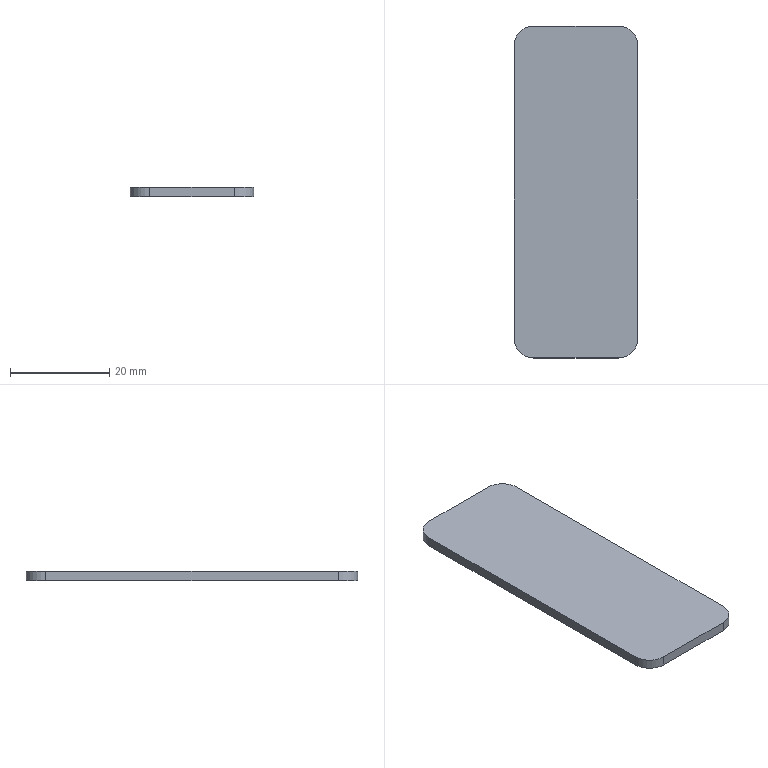Part | STEP file | X77-08306 | 1 solid | 10 faces | box 25 x 67 x 2 mm | volume 3323 mm3 | plane 6 | cylinder 4 | commonest cylinder face diameters 8 x4
STEP:
#1=CARTESIAN_POINT('',(-8.5,622.876,0.));
#2=VERTEX_POINT('',#1);
#3=CARTESIAN_POINT('',(-12.5,618.876,0.));
#4=VERTEX_POINT('',#3);
#5=CARTESIAN_POINT('',(-8.5,618.876,0.));
#6=DIRECTION('',(0.,0.,1.));
#7=DIRECTION('',(1.,0.,0.));
#8=AXIS2_PLACEMENT_3D('',#5,#6,#7);
#9=CIRCLE('',#8,4.);
#10=EDGE_CURVE('',#2,#4,#9,.T.);
#11=ORIENTED_EDGE('',*,*,#10,.T.);
#12=CARTESIAN_POINT('',(-12.5,618.876,2.));
#13=VERTEX_POINT('',#12);
#14=CARTESIAN_POINT('',(-12.5,618.876,2.));
#15=DIRECTION('',(0.,0.,-1.));
#16=VECTOR('',#15,1000.);
#17=LINE('',#14,#16);
#18=EDGE_CURVE('',#13,#4,#17,.T.);
#19=ORIENTED_EDGE('',*,*,#18,.F.);
#20=CARTESIAN_POINT('',(-8.5,622.876,2.));
#21=VERTEX_POINT('',#20);
#22=CARTESIAN_POINT('',(-8.5,618.876,2.));
#23=DIRECTION('',(0.,0.,1.));
#24=DIRECTION('',(1.,0.,0.));
#25=AXIS2_PLACEMENT_3D('',#22,#23,#24);
#26=CIRCLE('',#25,4.);
#27=EDGE_CURVE('',#21,#13,#26,.T.);
#28=ORIENTED_EDGE('',*,*,#27,.F.);
#29=CARTESIAN_POINT('',(-8.5,622.876,2.));
#30=DIRECTION('',(0.,0.,-1.));
#31=VECTOR('',#30,1000.);
#32=LINE('',#29,#31);
#33=EDGE_CURVE('',#21,#2,#32,.T.);
#34=ORIENTED_EDGE('',*,*,#33,.T.);
#35=EDGE_LOOP('',(#11,#19,#28,#34));
#36=FACE_OUTER_BOUND('',#35,.T.);
#37=CARTESIAN_POINT('',(-8.5,618.876,2.));
#38=DIRECTION('',(0.,0.,-1.));
#39=DIRECTION('',(-1.,0.,0.));
#40=AXIS2_PLACEMENT_3D('',#37,#38,#39);
#41=CYLINDRICAL_SURFACE('',#40,4.);
#42=ADVANCED_FACE('',(#36),#41,.T.);
#43=CARTESIAN_POINT('',(-12.5,559.876,0.));
#44=VERTEX_POINT('',#43);
#45=CARTESIAN_POINT('',(-12.5,618.876,0.));
#46=DIRECTION('',(0.,-1.,0.));
#47=VECTOR('',#46,1000.);
#48=LINE('',#45,#47);
#49=EDGE_CURVE('',#4,#44,#48,.T.);
#50=ORIENTED_EDGE('',*,*,#49,.T.);
#51=CARTESIAN_POINT('',(-12.5,559.876,2.));
#52=VERTEX_POINT('',#51);
#53=CARTESIAN_POINT('',(-12.5,559.876,2.));
#54=DIRECTION('',(0.,0.,-1.));
#55=VECTOR('',#54,1000.);
#56=LINE('',#53,#55);
#57=EDGE_CURVE('',#52,#44,#56,.T.);
#58=ORIENTED_EDGE('',*,*,#57,.F.);
#59=CARTESIAN_POINT('',(-12.5,618.876,2.));
#60=DIRECTION('',(0.,-1.,0.));
#61=VECTOR('',#60,1000.);
#62=LINE('',#59,#61);
#63=EDGE_CURVE('',#13,#52,#62,.T.);
#64=ORIENTED_EDGE('',*,*,#63,.F.);
#65=ORIENTED_EDGE('',*,*,#18,.T.);
#66=EDGE_LOOP('',(#50,#58,#64,#65));
#67=FACE_OUTER_BOUND('',#66,.T.);
#68=CARTESIAN_POINT('',(-12.5,618.876,2.));
#69=DIRECTION('',(1.,0.,0.));
#70=DIRECTION('',(0.,0.,-1.));
#71=AXIS2_PLACEMENT_3D('',#68,#69,#70);
#72=PLANE('',#71);
#73=ADVANCED_FACE('',(#67),#72,.F.);
#74=CARTESIAN_POINT('',(-8.5,555.876,0.));
#75=VERTEX_POINT('',#74);
#76=CARTESIAN_POINT('',(-8.5,559.876,0.));
#77=DIRECTION('',(0.,0.,1.));
#78=DIRECTION('',(1.,0.,0.));
#79=AXIS2_PLACEMENT_3D('',#76,#77,#78);
#80=CIRCLE('',#79,4.);
#81=EDGE_CURVE('',#44,#75,#80,.T.);
#82=ORIENTED_EDGE('',*,*,#81,.T.);
#83=CARTESIAN_POINT('',(-8.5,555.876,2.));
#84=VERTEX_POINT('',#83);
#85=CARTESIAN_POINT('',(-8.5,555.876,2.));
#86=DIRECTION('',(0.,0.,-1.));
#87=VECTOR('',#86,1000.);
#88=LINE('',#85,#87);
#89=EDGE_CURVE('',#84,#75,#88,.T.);
#90=ORIENTED_EDGE('',*,*,#89,.F.);
#91=CARTESIAN_POINT('',(-8.5,559.876,2.));
#92=DIRECTION('',(0.,0.,1.));
#93=DIRECTION('',(1.,0.,0.));
#94=AXIS2_PLACEMENT_3D('',#91,#92,#93);
#95=CIRCLE('',#94,4.);
#96=EDGE_CURVE('',#52,#84,#95,.T.);
#97=ORIENTED_EDGE('',*,*,#96,.F.);
#98=ORIENTED_EDGE('',*,*,#57,.T.);
#99=EDGE_LOOP('',(#82,#90,#97,#98));
#100=FACE_OUTER_BOUND('',#99,.T.);
#101=CARTESIAN_POINT('',(-8.5,559.876,2.));
#102=DIRECTION('',(0.,0.,-1.));
#103=DIRECTION('',(-1.,0.,0.));
#104=AXIS2_PLACEMENT_3D('',#101,#102,#103);
#105=CYLINDRICAL_SURFACE('',#104,4.);
#106=ADVANCED_FACE('',(#100),#105,.T.);
#107=CARTESIAN_POINT('',(8.5,555.876,0.));
#108=VERTEX_POINT('',#107);
#109=CARTESIAN_POINT('',(-8.5,555.876,0.));
#110=DIRECTION('',(1.,0.,0.));
#111=VECTOR('',#110,1000.);
#112=LINE('',#109,#111);
#113=EDGE_CURVE('',#75,#108,#112,.T.);
#114=ORIENTED_EDGE('',*,*,#113,.T.);
#115=CARTESIAN_POINT('',(8.5,555.876,2.));
#116=VERTEX_POINT('',#115);
#117=CARTESIAN_POINT('',(8.5,555.876,2.));
#118=DIRECTION('',(0.,0.,-1.));
#119=VECTOR('',#118,1000.);
#120=LINE('',#117,#119);
#121=EDGE_CURVE('',#116,#108,#120,.T.);
#122=ORIENTED_EDGE('',*,*,#121,.F.);
#123=CARTESIAN_POINT('',(-8.5,555.876,2.));
#124=DIRECTION('',(1.,0.,0.));
#125=VECTOR('',#124,1000.);
#126=LINE('',#123,#125);
#127=EDGE_CURVE('',#84,#116,#126,.T.);
#128=ORIENTED_EDGE('',*,*,#127,.F.);
#129=ORIENTED_EDGE('',*,*,#89,.T.);
#130=EDGE_LOOP('',(#114,#122,#128,#129));
#131=FACE_OUTER_BOUND('',#130,.T.);
#132=CARTESIAN_POINT('',(-8.5,555.876,2.));
#133=DIRECTION('',(0.,1.,0.));
#134=DIRECTION('',(0.,0.,1.));
#135=AXIS2_PLACEMENT_3D('',#132,#133,#134);
#136=PLANE('',#135);
#137=ADVANCED_FACE('',(#131),#136,.F.);
#138=CARTESIAN_POINT('',(12.5,559.876,0.));
#139=VERTEX_POINT('',#138);
#140=CARTESIAN_POINT('',(8.5,559.876,0.));
#141=DIRECTION('',(0.,0.,1.));
#142=DIRECTION('',(1.,0.,0.));
#143=AXIS2_PLACEMENT_3D('',#140,#141,#142);
#144=CIRCLE('',#143,4.);
#145=EDGE_CURVE('',#108,#139,#144,.T.);
#146=ORIENTED_EDGE('',*,*,#145,.T.);
#147=CARTESIAN_POINT('',(12.5,559.876,2.));
#148=VERTEX_POINT('',#147);
#149=CARTESIAN_POINT('',(12.5,559.876,2.));
#150=DIRECTION('',(0.,0.,-1.));
#151=VECTOR('',#150,1000.);
#152=LINE('',#149,#151);
#153=EDGE_CURVE('',#148,#139,#152,.T.);
#154=ORIENTED_EDGE('',*,*,#153,.F.);
#155=CARTESIAN_POINT('',(8.5,559.876,2.));
#156=DIRECTION('',(0.,0.,1.));
#157=DIRECTION('',(1.,0.,0.));
#158=AXIS2_PLACEMENT_3D('',#155,#156,#157);
#159=CIRCLE('',#158,4.);
#160=EDGE_CURVE('',#116,#148,#159,.T.);
#161=ORIENTED_EDGE('',*,*,#160,.F.);
#162=ORIENTED_EDGE('',*,*,#121,.T.);
#163=EDGE_LOOP('',(#146,#154,#161,#162));
#164=FACE_OUTER_BOUND('',#163,.T.);
#165=CARTESIAN_POINT('',(8.5,559.876,2.));
#166=DIRECTION('',(0.,0.,-1.));
#167=DIRECTION('',(-1.,0.,0.));
#168=AXIS2_PLACEMENT_3D('',#165,#166,#167);
#169=CYLINDRICAL_SURFACE('',#168,4.);
#170=ADVANCED_FACE('',(#164),#169,.T.);
#171=CARTESIAN_POINT('',(12.5,618.876,0.));
#172=VERTEX_POINT('',#171);
#173=CARTESIAN_POINT('',(12.5,559.876,0.));
#174=DIRECTION('',(0.,1.,0.));
#175=VECTOR('',#174,1000.);
#176=LINE('',#173,#175);
#177=EDGE_CURVE('',#139,#172,#176,.T.);
#178=ORIENTED_EDGE('',*,*,#177,.T.);
#179=CARTESIAN_POINT('',(12.5,618.876,2.));
#180=VERTEX_POINT('',#179);
#181=CARTESIAN_POINT('',(12.5,618.876,2.));
#182=DIRECTION('',(0.,0.,-1.));
#183=VECTOR('',#182,1000.);
#184=LINE('',#181,#183);
#185=EDGE_CURVE('',#180,#172,#184,.T.);
#186=ORIENTED_EDGE('',*,*,#185,.F.);
#187=CARTESIAN_POINT('',(12.5,559.876,2.));
#188=DIRECTION('',(0.,1.,0.));
#189=VECTOR('',#188,1000.);
#190=LINE('',#187,#189);
#191=EDGE_CURVE('',#148,#180,#190,.T.);
#192=ORIENTED_EDGE('',*,*,#191,.F.);
#193=ORIENTED_EDGE('',*,*,#153,.T.);
#194=EDGE_LOOP('',(#178,#186,#192,#193));
#195=FACE_OUTER_BOUND('',#194,.T.);
#196=CARTESIAN_POINT('',(12.5,559.876,2.));
#197=DIRECTION('',(-1.,0.,0.));
#198=DIRECTION('',(0.,0.,1.));
#199=AXIS2_PLACEMENT_3D('',#196,#197,#198);
#200=PLANE('',#199);
#201=ADVANCED_FACE('',(#195),#200,.F.);
#202=CARTESIAN_POINT('',(8.5,622.876,0.));
#203=VERTEX_POINT('',#202);
#204=CARTESIAN_POINT('',(8.5,618.876,0.));
#205=DIRECTION('',(0.,0.,1.));
#206=DIRECTION('',(1.,0.,0.));
#207=AXIS2_PLACEMENT_3D('',#204,#205,#206);
#208=CIRCLE('',#207,4.);
#209=EDGE_CURVE('',#172,#203,#208,.T.);
#210=ORIENTED_EDGE('',*,*,#209,.T.);
#211=CARTESIAN_POINT('',(8.5,622.876,2.));
#212=VERTEX_POINT('',#211);
#213=CARTESIAN_POINT('',(8.5,622.876,2.));
#214=DIRECTION('',(0.,0.,-1.));
#215=VECTOR('',#214,1000.);
#216=LINE('',#213,#215);
#217=EDGE_CURVE('',#212,#203,#216,.T.);
#218=ORIENTED_EDGE('',*,*,#217,.F.);
#219=CARTESIAN_POINT('',(8.5,618.876,2.));
#220=DIRECTION('',(0.,0.,1.));
#221=DIRECTION('',(1.,0.,0.));
#222=AXIS2_PLACEMENT_3D('',#219,#220,#221);
#223=CIRCLE('',#222,4.);
#224=EDGE_CURVE('',#180,#212,#223,.T.);
#225=ORIENTED_EDGE('',*,*,#224,.F.);
#226=ORIENTED_EDGE('',*,*,#185,.T.);
#227=EDGE_LOOP('',(#210,#218,#225,#226));
#228=FACE_OUTER_BOUND('',#227,.T.);
#229=CARTESIAN_POINT('',(8.5,618.876,2.));
#230=DIRECTION('',(0.,0.,-1.));
#231=DIRECTION('',(-1.,0.,0.));
#232=AXIS2_PLACEMENT_3D('',#229,#230,#231);
#233=CYLINDRICAL_SURFACE('',#232,4.);
#234=ADVANCED_FACE('',(#228),#233,.T.);
#235=CARTESIAN_POINT('',(8.5,622.876,0.));
#236=DIRECTION('',(-1.,0.,0.));
#237=VECTOR('',#236,1000.);
#238=LINE('',#235,#237);
#239=EDGE_CURVE('',#203,#2,#238,.T.);
#240=ORIENTED_EDGE('',*,*,#239,.T.);
#241=ORIENTED_EDGE('',*,*,#33,.F.);
#242=CARTESIAN_POINT('',(8.5,622.876,2.));
#243=DIRECTION('',(-1.,0.,0.));
#244=VECTOR('',#243,1000.);
#245=LINE('',#242,#244);
#246=EDGE_CURVE('',#212,#21,#245,.T.);
#247=ORIENTED_EDGE('',*,*,#246,.F.);
#248=ORIENTED_EDGE('',*,*,#217,.T.);
#249=EDGE_LOOP('',(#240,#241,#247,#248));
#250=FACE_OUTER_BOUND('',#249,.T.);
#251=CARTESIAN_POINT('',(8.5,622.876,2.));
#252=DIRECTION('',(0.,-1.,0.));
#253=DIRECTION('',(0.,0.,-1.));
#254=AXIS2_PLACEMENT_3D('',#251,#252,#253);
#255=PLANE('',#254);
#256=ADVANCED_FACE('',(#250),#255,.F.);
#257=ORIENTED_EDGE('',*,*,#27,.T.);
#258=ORIENTED_EDGE('',*,*,#63,.T.);
#259=ORIENTED_EDGE('',*,*,#96,.T.);
#260=ORIENTED_EDGE('',*,*,#127,.T.);
#261=ORIENTED_EDGE('',*,*,#160,.T.);
#262=ORIENTED_EDGE('',*,*,#191,.T.);
#263=ORIENTED_EDGE('',*,*,#224,.T.);
#264=ORIENTED_EDGE('',*,*,#246,.T.);
#265=EDGE_LOOP('',(#257,#258,#259,#260,#261,#262,#263,#264));
#266=FACE_OUTER_BOUND('',#265,.T.);
#267=CARTESIAN_POINT('',(-8.5,618.876,2.));
#268=DIRECTION('',(0.,0.,1.));
#269=DIRECTION('',(1.,0.,0.));
#270=AXIS2_PLACEMENT_3D('',#267,#268,#269);
#271=PLANE('',#270);
#272=ADVANCED_FACE('',(#266),#271,.T.);
#273=ORIENTED_EDGE('',*,*,#10,.F.);
#274=ORIENTED_EDGE('',*,*,#239,.F.);
#275=ORIENTED_EDGE('',*,*,#209,.F.);
#276=ORIENTED_EDGE('',*,*,#177,.F.);
#277=ORIENTED_EDGE('',*,*,#145,.F.);
#278=ORIENTED_EDGE('',*,*,#113,.F.);
#279=ORIENTED_EDGE('',*,*,#81,.F.);
#280=ORIENTED_EDGE('',*,*,#49,.F.);
#281=EDGE_LOOP('',(#273,#274,#275,#276,#277,#278,#279,#280));
#282=FACE_OUTER_BOUND('',#281,.T.);
#283=CARTESIAN_POINT('',(-8.5,618.876,0.));
#284=DIRECTION('',(0.,0.,1.));
#285=DIRECTION('',(1.,0.,0.));
#286=AXIS2_PLACEMENT_3D('',#283,#284,#285);
#287=PLANE('',#286);
#288=ADVANCED_FACE('',(#282),#287,.F.);
#289=CLOSED_SHELL('',(#42,#73,#106,#137,#170,#201,#234,#256,#272,#288));
#290=MANIFOLD_SOLID_BREP('',#289);
#291=CARTESIAN_POINT('',(0.,0.,0.));
#292=DIRECTION('',(0.,0.,1.));
#293=DIRECTION('',(1.,0.,0.));
#294=AXIS2_PLACEMENT_3D('',#291,#292,#293);
#295=(LENGTH_UNIT()NAMED_UNIT(*)SI_UNIT(.MILLI.,.METRE.));
#296=UNCERTAINTY_MEASURE_WITH_UNIT(LENGTH_MEASURE(0.00001),#295,'','');
#297=(NAMED_UNIT(*)PLANE_ANGLE_UNIT()SI_UNIT($,.RADIAN.));
#298=(NAMED_UNIT(*)SI_UNIT($,.STERADIAN.)SOLID_ANGLE_UNIT());
#299=(GEOMETRIC_REPRESENTATION_CONTEXT(3)GLOBAL_UNCERTAINTY_ASSIGNED_CONTEXT((#296))GLOBAL_UNIT_ASSIGNED_CONTEXT((#295,#297,#298))REPRESENTATION_CONTEXT('',''));
#300=ADVANCED_BREP_SHAPE_REPRESENTATION('',(#290,#294),#299);